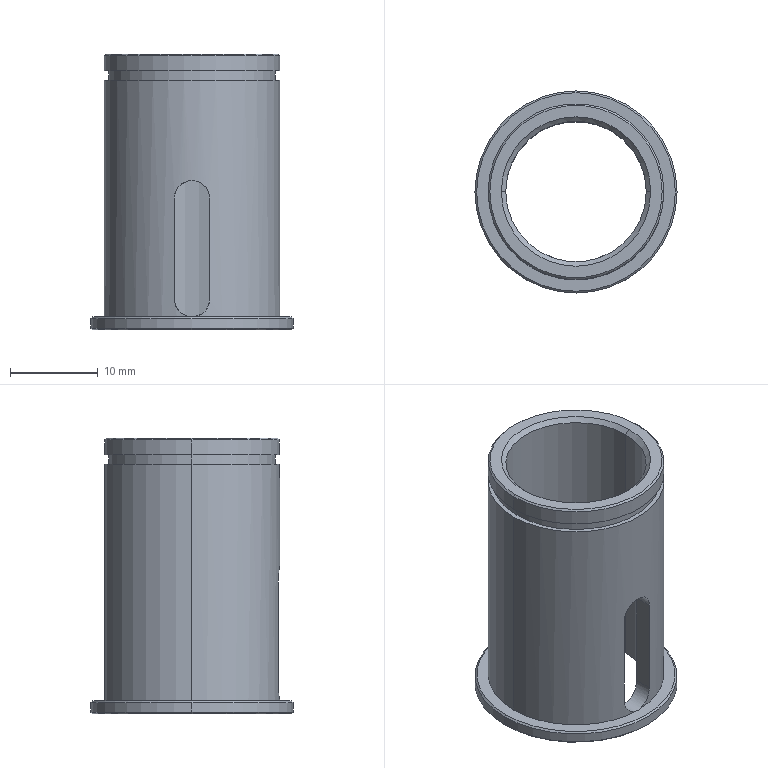Part | STEP file | Drive shaft sleeve | 1 solid | 30 faces | box 23 x 23 x 31.4 mm | volume 3535 mm3 | cylinder 13 | cone 10 | plane 7 | commonest cylinder face diameters 20 x4 4 x3 16 x2 19 x2 23 x2